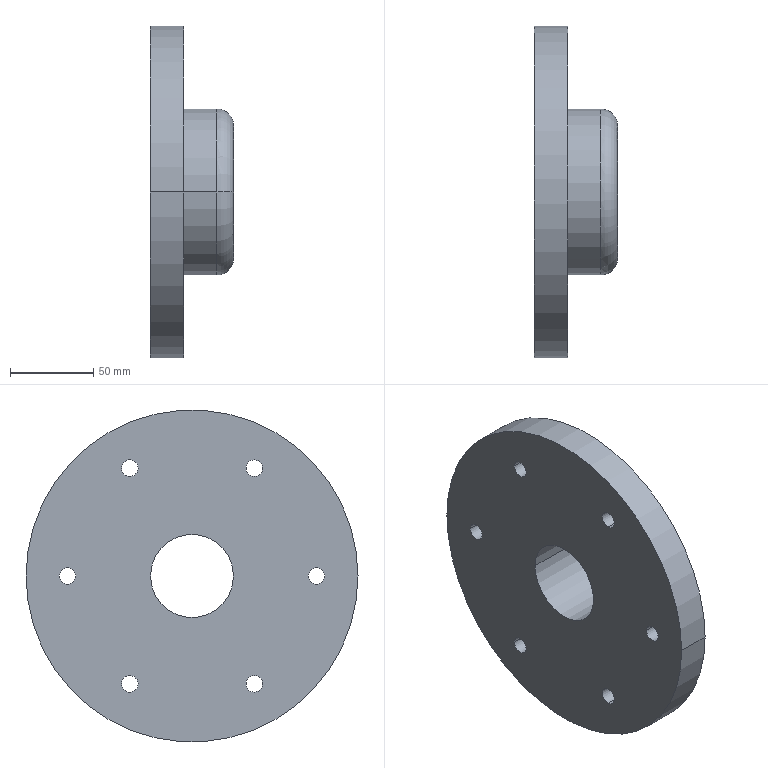Part | SolidWorks | features CirPattern 1, Fillet 1, ICE 1, Revolution 1 | 1 solid | 23 faces | box 50 x 200 x 200 mm | volume 749898 mm3 | cylinder 18 | plane 3 | torus 2 | commonest cylinder face diameters 10 x12 50 x2 100 x2 200 x2
STEP:
#1=CARTESIAN_POINT('',(40.,-50.,0.));
#2=VERTEX_POINT('',#1);
#3=CARTESIAN_POINT('',(40.,50.,0.));
#4=VERTEX_POINT('',#3);
#5=CARTESIAN_POINT('',(40.,0.,0.));
#6=DIRECTION('',(-1.,0.,0.));
#7=DIRECTION('',(0.,1.,0.));
#8=AXIS2_PLACEMENT_3D('',#5,#6,#7);
#9=CIRCLE('',#8,50.);
#10=EDGE_CURVE('',#2,#4,#9,.T.);
#11=ORIENTED_EDGE('',*,*,#10,.F.);
#12=CARTESIAN_POINT('',(50.,-40.,0.));
#13=VERTEX_POINT('',#12);
#14=CARTESIAN_POINT('',(40.,-40.,0.));
#15=DIRECTION('',(0.,0.,1.));
#16=DIRECTION('',(0.,-1.,0.));
#17=AXIS2_PLACEMENT_3D('',#14,#15,#16);
#18=CIRCLE('',#17,10.);
#19=EDGE_CURVE('',#2,#13,#18,.T.);
#20=ORIENTED_EDGE('',*,*,#19,.T.);
#21=CARTESIAN_POINT('',(50.,40.,0.));
#22=VERTEX_POINT('',#21);
#23=CARTESIAN_POINT('',(50.,0.,0.));
#24=DIRECTION('',(1.,0.,0.));
#25=DIRECTION('',(0.,1.,0.));
#26=AXIS2_PLACEMENT_3D('',#23,#24,#25);
#27=CIRCLE('',#26,40.);
#28=EDGE_CURVE('',#22,#13,#27,.T.);
#29=ORIENTED_EDGE('',*,*,#28,.F.);
#30=CARTESIAN_POINT('',(40.,40.,0.));
#31=DIRECTION('',(0.,0.,-1.));
#32=DIRECTION('',(-1.,0.,0.));
#33=AXIS2_PLACEMENT_3D('',#30,#31,#32);
#34=CIRCLE('',#33,10.);
#35=EDGE_CURVE('',#4,#22,#34,.T.);
#36=ORIENTED_EDGE('',*,*,#35,.F.);
#37=EDGE_LOOP('',(#11,#20,#29,#36));
#38=FACE_OUTER_BOUND('',#37,.T.);
#39=CARTESIAN_POINT('',(40.,0.,0.));
#40=DIRECTION('',(1.,0.,0.));
#41=DIRECTION('',(0.,1.,0.));
#42=AXIS2_PLACEMENT_3D('',#39,#40,#41);
#43=TOROIDAL_SURFACE('',#42,40.,10.);
#44=ADVANCED_FACE('',(#38),#43,.T.);
#45=CARTESIAN_POINT('',(0.,32.5,-64.952));
#46=VERTEX_POINT('',#45);
#47=CARTESIAN_POINT('',(0.,42.5,-64.952));
#48=VERTEX_POINT('',#47);
#49=CARTESIAN_POINT('',(0.,37.5,-64.952));
#50=DIRECTION('',(1.,0.,0.));
#51=DIRECTION('',(0.,-1.,0.));
#52=AXIS2_PLACEMENT_3D('',#49,#50,#51);
#53=CIRCLE('',#52,5.);
#54=EDGE_CURVE('',#46,#48,#53,.T.);
#55=ORIENTED_EDGE('',*,*,#54,.F.);
#56=CARTESIAN_POINT('',(20.,32.5,-64.952));
#57=VERTEX_POINT('',#56);
#58=CARTESIAN_POINT('',(-0.001,32.5,-64.952));
#59=DIRECTION('',(1.,0.,0.));
#60=VECTOR('',#59,1000.);
#61=LINE('',#58,#60);
#62=EDGE_CURVE('',#46,#57,#61,.T.);
#63=ORIENTED_EDGE('',*,*,#62,.T.);
#64=CARTESIAN_POINT('',(20.,42.5,-64.952));
#65=VERTEX_POINT('',#64);
#66=CARTESIAN_POINT('',(20.,37.5,-64.952));
#67=DIRECTION('',(1.,0.,0.));
#68=DIRECTION('',(0.,0.5,-0.866));
#69=AXIS2_PLACEMENT_3D('',#66,#67,#68);
#70=CIRCLE('',#69,5.);
#71=EDGE_CURVE('',#57,#65,#70,.T.);
#72=ORIENTED_EDGE('',*,*,#71,.T.);
#73=CARTESIAN_POINT('',(-0.001,42.5,-64.952));
#74=DIRECTION('',(1.,0.,0.));
#75=VECTOR('',#74,1000.);
#76=LINE('',#73,#75);
#77=EDGE_CURVE('',#48,#65,#76,.T.);
#78=ORIENTED_EDGE('',*,*,#77,.F.);
#79=EDGE_LOOP('',(#55,#63,#72,#78));
#80=FACE_OUTER_BOUND('',#79,.T.);
#81=CARTESIAN_POINT('',(-0.001,37.5,-64.952));
#82=DIRECTION('',(1.,0.,0.));
#83=DIRECTION('',(0.,1.,0.));
#84=AXIS2_PLACEMENT_3D('',#81,#82,#83);
#85=CYLINDRICAL_SURFACE('',#84,5.);
#86=ADVANCED_FACE('',(#80),#85,.F.);
#87=CARTESIAN_POINT('',(0.,-37.5,-59.952));
#88=VERTEX_POINT('',#87);
#89=CARTESIAN_POINT('',(0.,-37.5,-69.952));
#90=VERTEX_POINT('',#89);
#91=CARTESIAN_POINT('',(0.,-37.5,-64.952));
#92=DIRECTION('',(1.,0.,0.));
#93=DIRECTION('',(0.,-1.,0.));
#94=AXIS2_PLACEMENT_3D('',#91,#92,#93);
#95=CIRCLE('',#94,5.);
#96=EDGE_CURVE('',#88,#90,#95,.T.);
#97=ORIENTED_EDGE('',*,*,#96,.F.);
#98=CARTESIAN_POINT('',(20.,-37.5,-59.952));
#99=VERTEX_POINT('',#98);
#100=CARTESIAN_POINT('',(-0.001,-37.5,-59.952));
#101=DIRECTION('',(1.,0.,0.));
#102=VECTOR('',#101,1000.);
#103=LINE('',#100,#102);
#104=EDGE_CURVE('',#88,#99,#103,.T.);
#105=ORIENTED_EDGE('',*,*,#104,.T.);
#106=CARTESIAN_POINT('',(20.,-37.5,-69.952));
#107=VERTEX_POINT('',#106);
#108=CARTESIAN_POINT('',(20.,-37.5,-64.952));
#109=DIRECTION('',(1.,0.,0.));
#110=DIRECTION('',(0.,-0.5,-0.866));
#111=AXIS2_PLACEMENT_3D('',#108,#109,#110);
#112=CIRCLE('',#111,5.);
#113=EDGE_CURVE('',#99,#107,#112,.T.);
#114=ORIENTED_EDGE('',*,*,#113,.T.);
#115=CARTESIAN_POINT('',(-0.001,-37.5,-69.952));
#116=DIRECTION('',(1.,0.,0.));
#117=VECTOR('',#116,1000.);
#118=LINE('',#115,#117);
#119=EDGE_CURVE('',#90,#107,#118,.T.);
#120=ORIENTED_EDGE('',*,*,#119,.F.);
#121=EDGE_LOOP('',(#97,#105,#114,#120));
#122=FACE_OUTER_BOUND('',#121,.T.);
#123=CARTESIAN_POINT('',(-0.001,-37.5,-64.952));
#124=DIRECTION('',(1.,0.,0.));
#125=DIRECTION('',(0.,0.,-1.));
#126=AXIS2_PLACEMENT_3D('',#123,#124,#125);
#127=CYLINDRICAL_SURFACE('',#126,5.);
#128=ADVANCED_FACE('',(#122),#127,.F.);
#129=CARTESIAN_POINT('',(0.,-80.,0.));
#130=VERTEX_POINT('',#129);
#131=CARTESIAN_POINT('',(0.,-70.,0.));
#132=VERTEX_POINT('',#131);
#133=CARTESIAN_POINT('',(0.,-75.,0.));
#134=DIRECTION('',(1.,0.,0.));
#135=DIRECTION('',(0.,-1.,0.));
#136=AXIS2_PLACEMENT_3D('',#133,#134,#135);
#137=CIRCLE('',#136,5.);
#138=EDGE_CURVE('',#130,#132,#137,.T.);
#139=ORIENTED_EDGE('',*,*,#138,.F.);
#140=CARTESIAN_POINT('',(20.,-80.,0.));
#141=VERTEX_POINT('',#140);
#142=CARTESIAN_POINT('',(-0.001,-80.,0.));
#143=DIRECTION('',(1.,0.,0.));
#144=VECTOR('',#143,1000.);
#145=LINE('',#142,#144);
#146=EDGE_CURVE('',#130,#141,#145,.T.);
#147=ORIENTED_EDGE('',*,*,#146,.T.);
#148=CARTESIAN_POINT('',(20.,-70.,0.));
#149=VERTEX_POINT('',#148);
#150=CARTESIAN_POINT('',(20.,-75.,0.));
#151=DIRECTION('',(1.,0.,0.));
#152=DIRECTION('',(0.,-1.,0.));
#153=AXIS2_PLACEMENT_3D('',#150,#151,#152);
#154=CIRCLE('',#153,5.);
#155=EDGE_CURVE('',#141,#149,#154,.T.);
#156=ORIENTED_EDGE('',*,*,#155,.T.);
#157=CARTESIAN_POINT('',(-0.001,-70.,0.));
#158=DIRECTION('',(1.,0.,0.));
#159=VECTOR('',#158,1000.);
#160=LINE('',#157,#159);
#161=EDGE_CURVE('',#132,#149,#160,.T.);
#162=ORIENTED_EDGE('',*,*,#161,.F.);
#163=EDGE_LOOP('',(#139,#147,#156,#162));
#164=FACE_OUTER_BOUND('',#163,.T.);
#165=CARTESIAN_POINT('',(-0.001,-75.,0.));
#166=DIRECTION('',(1.,0.,0.));
#167=DIRECTION('',(0.,1.,0.));
#168=AXIS2_PLACEMENT_3D('',#165,#166,#167);
#169=CYLINDRICAL_SURFACE('',#168,5.);
#170=ADVANCED_FACE('',(#164),#169,.F.);
#171=CARTESIAN_POINT('',(0.,-37.5,69.952));
#172=VERTEX_POINT('',#171);
#173=CARTESIAN_POINT('',(0.,-37.5,59.952));
#174=VERTEX_POINT('',#173);
#175=CARTESIAN_POINT('',(0.,-37.5,64.952));
#176=DIRECTION('',(1.,0.,0.));
#177=DIRECTION('',(0.,-1.,0.));
#178=AXIS2_PLACEMENT_3D('',#175,#176,#177);
#179=CIRCLE('',#178,5.);
#180=EDGE_CURVE('',#172,#174,#179,.T.);
#181=ORIENTED_EDGE('',*,*,#180,.F.);
#182=CARTESIAN_POINT('',(20.,-37.5,69.952));
#183=VERTEX_POINT('',#182);
#184=CARTESIAN_POINT('',(-0.001,-37.5,69.952));
#185=DIRECTION('',(1.,0.,0.));
#186=VECTOR('',#185,1000.);
#187=LINE('',#184,#186);
#188=EDGE_CURVE('',#172,#183,#187,.T.);
#189=ORIENTED_EDGE('',*,*,#188,.T.);
#190=CARTESIAN_POINT('',(20.,-37.5,59.952));
#191=VERTEX_POINT('',#190);
#192=CARTESIAN_POINT('',(20.,-37.5,64.952));
#193=DIRECTION('',(1.,0.,0.));
#194=DIRECTION('',(0.,-0.5,0.866));
#195=AXIS2_PLACEMENT_3D('',#192,#193,#194);
#196=CIRCLE('',#195,5.);
#197=EDGE_CURVE('',#183,#191,#196,.T.);
#198=ORIENTED_EDGE('',*,*,#197,.T.);
#199=CARTESIAN_POINT('',(-0.001,-37.5,59.952));
#200=DIRECTION('',(1.,0.,0.));
#201=VECTOR('',#200,1000.);
#202=LINE('',#199,#201);
#203=EDGE_CURVE('',#174,#191,#202,.T.);
#204=ORIENTED_EDGE('',*,*,#203,.F.);
#205=EDGE_LOOP('',(#181,#189,#198,#204));
#206=FACE_OUTER_BOUND('',#205,.T.);
#207=CARTESIAN_POINT('',(-0.001,-37.5,64.952));
#208=DIRECTION('',(1.,0.,0.));
#209=DIRECTION('',(0.,0.,-1.));
#210=AXIS2_PLACEMENT_3D('',#207,#208,#209);
#211=CYLINDRICAL_SURFACE('',#210,5.);
#212=ADVANCED_FACE('',(#206),#211,.F.);
#213=CARTESIAN_POINT('',(0.,32.5,64.952));
#214=VERTEX_POINT('',#213);
#215=CARTESIAN_POINT('',(0.,42.5,64.952));
#216=VERTEX_POINT('',#215);
#217=CARTESIAN_POINT('',(0.,37.5,64.952));
#218=DIRECTION('',(1.,0.,0.));
#219=DIRECTION('',(0.,-1.,0.));
#220=AXIS2_PLACEMENT_3D('',#217,#218,#219);
#221=CIRCLE('',#220,5.);
#222=EDGE_CURVE('',#214,#216,#221,.T.);
#223=ORIENTED_EDGE('',*,*,#222,.F.);
#224=CARTESIAN_POINT('',(20.,32.5,64.952));
#225=VERTEX_POINT('',#224);
#226=CARTESIAN_POINT('',(-0.001,32.5,64.952));
#227=DIRECTION('',(1.,0.,0.));
#228=VECTOR('',#227,1000.);
#229=LINE('',#226,#228);
#230=EDGE_CURVE('',#214,#225,#229,.T.);
#231=ORIENTED_EDGE('',*,*,#230,.T.);
#232=CARTESIAN_POINT('',(20.,42.5,64.952));
#233=VERTEX_POINT('',#232);
#234=CARTESIAN_POINT('',(20.,37.5,64.952));
#235=DIRECTION('',(1.,0.,0.));
#236=DIRECTION('',(0.,0.5,0.866));
#237=AXIS2_PLACEMENT_3D('',#234,#235,#236);
#238=CIRCLE('',#237,5.);
#239=EDGE_CURVE('',#225,#233,#238,.T.);
#240=ORIENTED_EDGE('',*,*,#239,.T.);
#241=CARTESIAN_POINT('',(-0.001,42.5,64.952));
#242=DIRECTION('',(1.,0.,0.));
#243=VECTOR('',#242,1000.);
#244=LINE('',#241,#243);
#245=EDGE_CURVE('',#216,#233,#244,.T.);
#246=ORIENTED_EDGE('',*,*,#245,.F.);
#247=EDGE_LOOP('',(#223,#231,#240,#246));
#248=FACE_OUTER_BOUND('',#247,.T.);
#249=CARTESIAN_POINT('',(-0.001,37.5,64.952));
#250=DIRECTION('',(1.,0.,0.));
#251=DIRECTION('',(0.,1.,0.));
#252=AXIS2_PLACEMENT_3D('',#249,#250,#251);
#253=CYLINDRICAL_SURFACE('',#252,5.);
#254=ADVANCED_FACE('',(#248),#253,.F.);
#255=CARTESIAN_POINT('',(0.,70.,0.));
#256=VERTEX_POINT('',#255);
#257=CARTESIAN_POINT('',(0.,80.,0.));
#258=VERTEX_POINT('',#257);
#259=CARTESIAN_POINT('',(0.,75.,0.));
#260=DIRECTION('',(1.,0.,0.));
#261=DIRECTION('',(0.,-1.,0.));
#262=AXIS2_PLACEMENT_3D('',#259,#260,#261);
#263=CIRCLE('',#262,5.);
#264=EDGE_CURVE('',#256,#258,#263,.T.);
#265=ORIENTED_EDGE('',*,*,#264,.F.);
#266=CARTESIAN_POINT('',(20.,70.,0.));
#267=VERTEX_POINT('',#266);
#268=CARTESIAN_POINT('',(-0.001,70.,0.));
#269=DIRECTION('',(1.,0.,0.));
#270=VECTOR('',#269,1000.);
#271=LINE('',#268,#270);
#272=EDGE_CURVE('',#256,#267,#271,.T.);
#273=ORIENTED_EDGE('',*,*,#272,.T.);
#274=CARTESIAN_POINT('',(20.,80.,0.));
#275=VERTEX_POINT('',#274);
#276=CARTESIAN_POINT('',(20.,75.,0.));
#277=DIRECTION('',(1.,0.,0.));
#278=DIRECTION('',(0.,1.,0.));
#279=AXIS2_PLACEMENT_3D('',#276,#277,#278);
#280=CIRCLE('',#279,5.);
#281=EDGE_CURVE('',#267,#275,#280,.T.);
#282=ORIENTED_EDGE('',*,*,#281,.T.);
#283=CARTESIAN_POINT('',(-0.001,80.,0.));
#284=DIRECTION('',(1.,0.,0.));
#285=VECTOR('',#284,1000.);
#286=LINE('',#283,#285);
#287=EDGE_CURVE('',#258,#275,#286,.T.);
#288=ORIENTED_EDGE('',*,*,#287,.F.);
#289=EDGE_LOOP('',(#265,#273,#282,#288));
#290=FACE_OUTER_BOUND('',#289,.T.);
#291=CARTESIAN_POINT('',(-0.001,75.,0.));
#292=DIRECTION('',(1.,0.,0.));
#293=DIRECTION('',(0.,1.,0.));
#294=AXIS2_PLACEMENT_3D('',#291,#292,#293);
#295=CYLINDRICAL_SURFACE('',#294,5.);
#296=ADVANCED_FACE('',(#290),#295,.F.);
#297=CARTESIAN_POINT('',(0.,-25.,0.));
#298=VERTEX_POINT('',#297);
#299=CARTESIAN_POINT('',(0.,25.,0.));
#300=VERTEX_POINT('',#299);
#301=CARTESIAN_POINT('',(0.,0.,0.));
#302=DIRECTION('',(1.,0.,0.));
#303=DIRECTION('',(0.,1.,0.));
#304=AXIS2_PLACEMENT_3D('',#301,#302,#303);
#305=CIRCLE('',#304,25.);
#306=EDGE_CURVE('',#298,#300,#305,.T.);
#307=ORIENTED_EDGE('',*,*,#306,.F.);
#308=CARTESIAN_POINT('',(50.,-25.,0.));
#309=VERTEX_POINT('',#308);
#310=CARTESIAN_POINT('',(113.214,-25.,0.));
#311=DIRECTION('',(1.,0.,0.));
#312=VECTOR('',#311,1000.);
#313=LINE('',#310,#312);
#314=EDGE_CURVE('',#298,#309,#313,.T.);
#315=ORIENTED_EDGE('',*,*,#314,.T.);
#316=CARTESIAN_POINT('',(50.,25.,0.));
#317=VERTEX_POINT('',#316);
#318=CARTESIAN_POINT('',(50.,0.,0.));
#319=DIRECTION('',(1.,0.,0.));
#320=DIRECTION('',(0.,1.,0.));
#321=AXIS2_PLACEMENT_3D('',#318,#319,#320);
#322=CIRCLE('',#321,25.);
#323=EDGE_CURVE('',#309,#317,#322,.T.);
#324=ORIENTED_EDGE('',*,*,#323,.T.);
#325=CARTESIAN_POINT('',(113.214,25.,0.));
#326=DIRECTION('',(1.,0.,0.));
#327=VECTOR('',#326,1000.);
#328=LINE('',#325,#327);
#329=EDGE_CURVE('',#300,#317,#328,.T.);
#330=ORIENTED_EDGE('',*,*,#329,.F.);
#331=EDGE_LOOP('',(#307,#315,#324,#330));
#332=FACE_OUTER_BOUND('',#331,.T.);
#333=CARTESIAN_POINT('',(113.214,0.,0.));
#334=DIRECTION('',(1.,0.,0.));
#335=DIRECTION('',(0.,1.,0.));
#336=AXIS2_PLACEMENT_3D('',#333,#334,#335);
#337=CYLINDRICAL_SURFACE('',#336,25.);
#338=ADVANCED_FACE('',(#332),#337,.F.);
#339=CARTESIAN_POINT('',(20.,50.,0.));
#340=VERTEX_POINT('',#339);
#341=CARTESIAN_POINT('',(20.,-50.,0.));
#342=VERTEX_POINT('',#341);
#343=CARTESIAN_POINT('',(20.,0.,0.));
#344=DIRECTION('',(1.,0.,0.));
#345=DIRECTION('',(0.,1.,0.));
#346=AXIS2_PLACEMENT_3D('',#343,#344,#345);
#347=CIRCLE('',#346,50.);
#348=EDGE_CURVE('',#340,#342,#347,.T.);
#349=ORIENTED_EDGE('',*,*,#348,.T.);
#350=CARTESIAN_POINT('',(113.214,-50.,0.));
#351=DIRECTION('',(1.,0.,0.));
#352=VECTOR('',#351,1000.);
#353=LINE('',#350,#352);
#354=EDGE_CURVE('',#342,#2,#353,.T.);
#355=ORIENTED_EDGE('',*,*,#354,.T.);
#356=ORIENTED_EDGE('',*,*,#10,.T.);
#357=CARTESIAN_POINT('',(113.214,50.,0.));
#358=DIRECTION('',(1.,0.,0.));
#359=VECTOR('',#358,1000.);
#360=LINE('',#357,#359);
#361=EDGE_CURVE('',#340,#4,#360,.T.);
#362=ORIENTED_EDGE('',*,*,#361,.F.);
#363=EDGE_LOOP('',(#349,#355,#356,#362));
#364=FACE_OUTER_BOUND('',#363,.T.);
#365=CARTESIAN_POINT('',(113.214,0.,0.));
#366=DIRECTION('',(1.,0.,0.));
#367=DIRECTION('',(0.,1.,0.));
#368=AXIS2_PLACEMENT_3D('',#365,#366,#367);
#369=CYLINDRICAL_SURFACE('',#368,50.);
#370=ADVANCED_FACE('',(#364),#369,.T.);
#371=CARTESIAN_POINT('',(0.,100.,0.));
#372=VERTEX_POINT('',#371);
#373=CARTESIAN_POINT('',(0.,-100.,0.));
#374=VERTEX_POINT('',#373);
#375=CARTESIAN_POINT('',(0.,0.,0.));
#376=DIRECTION('',(1.,0.,0.));
#377=DIRECTION('',(0.,1.,0.));
#378=AXIS2_PLACEMENT_3D('',#375,#376,#377);
#379=CIRCLE('',#378,100.);
#380=EDGE_CURVE('',#372,#374,#379,.T.);
#381=ORIENTED_EDGE('',*,*,#380,.T.);
#382=CARTESIAN_POINT('',(20.,-100.,0.));
#383=VERTEX_POINT('',#382);
#384=CARTESIAN_POINT('',(113.214,-100.,0.));
#385=DIRECTION('',(1.,0.,0.));
#386=VECTOR('',#385,1000.);
#387=LINE('',#384,#386);
#388=EDGE_CURVE('',#374,#383,#387,.T.);
#389=ORIENTED_EDGE('',*,*,#388,.T.);
#390=CARTESIAN_POINT('',(20.,100.,0.));
#391=VERTEX_POINT('',#390);
#392=CARTESIAN_POINT('',(20.,0.,0.));
#393=DIRECTION('',(1.,0.,0.));
#394=DIRECTION('',(0.,1.,0.));
#395=AXIS2_PLACEMENT_3D('',#392,#393,#394);
#396=CIRCLE('',#395,100.);
#397=EDGE_CURVE('',#391,#383,#396,.T.);
#398=ORIENTED_EDGE('',*,*,#397,.F.);
#399=CARTESIAN_POINT('',(113.214,100.,0.));
#400=DIRECTION('',(1.,0.,0.));
#401=VECTOR('',#400,1000.);
#402=LINE('',#399,#401);
#403=EDGE_CURVE('',#372,#391,#402,.T.);
#404=ORIENTED_EDGE('',*,*,#403,.F.);
#405=EDGE_LOOP('',(#381,#389,#398,#404));
#406=FACE_OUTER_BOUND('',#405,.T.);
#407=CARTESIAN_POINT('',(113.214,0.,0.));
#408=DIRECTION('',(1.,0.,0.));
#409=DIRECTION('',(0.,1.,0.));
#410=AXIS2_PLACEMENT_3D('',#407,#408,#409);
#411=CYLINDRICAL_SURFACE('',#410,100.);
#412=ADVANCED_FACE('',(#406),#411,.T.);
#413=ORIENTED_EDGE('',*,*,#388,.F.);
#414=CARTESIAN_POINT('',(0.,0.,0.));
#415=DIRECTION('',(1.,0.,0.));
#416=DIRECTION('',(0.,1.,0.));
#417=AXIS2_PLACEMENT_3D('',#414,#415,#416);
#418=CIRCLE('',#417,100.);
#419=EDGE_CURVE('',#374,#372,#418,.T.);
#420=ORIENTED_EDGE('',*,*,#419,.T.);
#421=ORIENTED_EDGE('',*,*,#403,.T.);
#422=CARTESIAN_POINT('',(20.,0.,0.));
#423=DIRECTION('',(1.,0.,0.));
#424=DIRECTION('',(0.,1.,0.));
#425=AXIS2_PLACEMENT_3D('',#422,#423,#424);
#426=CIRCLE('',#425,100.);
#427=EDGE_CURVE('',#383,#391,#426,.T.);
#428=ORIENTED_EDGE('',*,*,#427,.F.);
#429=EDGE_LOOP('',(#413,#420,#421,#428));
#430=FACE_OUTER_BOUND('',#429,.T.);
#431=CARTESIAN_POINT('',(113.214,0.,0.));
#432=DIRECTION('',(1.,0.,0.));
#433=DIRECTION('',(0.,1.,0.));
#434=AXIS2_PLACEMENT_3D('',#431,#432,#433);
#435=CYLINDRICAL_SURFACE('',#434,100.);
#436=ADVANCED_FACE('',(#430),#435,.T.);
#437=CARTESIAN_POINT('',(20.,37.5,-64.952));
#438=DIRECTION('',(1.,0.,0.));
#439=DIRECTION('',(0.,0.5,-0.866));
#440=AXIS2_PLACEMENT_3D('',#437,#438,#439);
#441=CIRCLE('',#440,5.);
#442=EDGE_CURVE('',#65,#57,#441,.T.);
#443=ORIENTED_EDGE('',*,*,#442,.F.);
#444=ORIENTED_EDGE('',*,*,#71,.F.);
#445=EDGE_LOOP('',(#443,#444));
#446=FACE_BOUND('',#445,.T.);
#447=CARTESIAN_POINT('',(20.,-37.5,-64.952));
#448=DIRECTION('',(1.,0.,0.));
#449=DIRECTION('',(0.,-0.5,-0.866));
#450=AXIS2_PLACEMENT_3D('',#447,#448,#449);
#451=CIRCLE('',#450,5.);
#452=EDGE_CURVE('',#107,#99,#451,.T.);
#453=ORIENTED_EDGE('',*,*,#452,.F.);
#454=ORIENTED_EDGE('',*,*,#113,.F.);
#455=EDGE_LOOP('',(#453,#454));
#456=FACE_BOUND('',#455,.T.);
#457=CARTESIAN_POINT('',(20.,-75.,0.));
#458=DIRECTION('',(1.,0.,0.));
#459=DIRECTION('',(0.,-1.,0.));
#460=AXIS2_PLACEMENT_3D('',#457,#458,#459);
#461=CIRCLE('',#460,5.);
#462=EDGE_CURVE('',#149,#141,#461,.T.);
#463=ORIENTED_EDGE('',*,*,#462,.F.);
#464=ORIENTED_EDGE('',*,*,#155,.F.);
#465=EDGE_LOOP('',(#463,#464));
#466=FACE_BOUND('',#465,.T.);
#467=CARTESIAN_POINT('',(20.,-37.5,64.952));
#468=DIRECTION('',(1.,0.,0.));
#469=DIRECTION('',(0.,-0.5,0.866));
#470=AXIS2_PLACEMENT_3D('',#467,#468,#469);
#471=CIRCLE('',#470,5.);
#472=EDGE_CURVE('',#191,#183,#471,.T.);
#473=ORIENTED_EDGE('',*,*,#472,.F.);
#474=ORIENTED_EDGE('',*,*,#197,.F.);
#475=EDGE_LOOP('',(#473,#474));
#476=FACE_BOUND('',#475,.T.);
#477=CARTESIAN_POINT('',(20.,37.5,64.952));
#478=DIRECTION('',(1.,0.,0.));
#479=DIRECTION('',(0.,0.5,0.866));
#480=AXIS2_PLACEMENT_3D('',#477,#478,#479);
#481=CIRCLE('',#480,5.);
#482=EDGE_CURVE('',#233,#225,#481,.T.);
#483=ORIENTED_EDGE('',*,*,#482,.F.);
#484=ORIENTED_EDGE('',*,*,#239,.F.);
#485=EDGE_LOOP('',(#483,#484));
#486=FACE_BOUND('',#485,.T.);
#487=CARTESIAN_POINT('',(20.,75.,0.));
#488=DIRECTION('',(1.,0.,0.));
#489=DIRECTION('',(0.,1.,0.));
#490=AXIS2_PLACEMENT_3D('',#487,#488,#489);
#491=CIRCLE('',#490,5.);
#492=EDGE_CURVE('',#275,#267,#491,.T.);
#493=ORIENTED_EDGE('',*,*,#492,.F.);
#494=ORIENTED_EDGE('',*,*,#281,.F.);
#495=EDGE_LOOP('',(#493,#494));
#496=FACE_BOUND('',#495,.T.);
#497=ORIENTED_EDGE('',*,*,#397,.T.);
#498=ORIENTED_EDGE('',*,*,#427,.T.);
#499=EDGE_LOOP('',(#497,#498));
#500=FACE_OUTER_BOUND('',#499,.T.);
#501=ORIENTED_EDGE('',*,*,#348,.F.);
#502=CARTESIAN_POINT('',(20.,0.,0.));
#503=DIRECTION('',(1.,0.,0.));
#504=DIRECTION('',(0.,1.,0.));
#505=AXIS2_PLACEMENT_3D('',#502,#503,#504);
#506=CIRCLE('',#505,50.);
#507=EDGE_CURVE('',#342,#340,#506,.T.);
#508=ORIENTED_EDGE('',*,*,#507,.F.);
#509=EDGE_LOOP('',(#501,#508));
#510=FACE_BOUND('',#509,.T.);
#511=CARTESIAN_POINT('',(20.,100.,0.));
#512=DIRECTION('',(1.,0.,0.));
#513=DIRECTION('',(0.,1.,0.));
#514=AXIS2_PLACEMENT_3D('',#511,#512,#513);
#515=PLANE('',#514);
#516=ADVANCED_FACE('',(#446,#456,#466,#476,#486,#496,#500,#510),#515,.T.);
#517=ORIENTED_EDGE('',*,*,#354,.F.);
#518=ORIENTED_EDGE('',*,*,#507,.T.);
#519=ORIENTED_EDGE('',*,*,#361,.T.);
#520=CARTESIAN_POINT('',(40.,0.,0.));
#521=DIRECTION('',(-1.,0.,0.));
#522=DIRECTION('',(0.,1.,0.));
#523=AXIS2_PLACEMENT_3D('',#520,#521,#522);
#524=CIRCLE('',#523,50.);
#525=EDGE_CURVE('',#4,#2,#524,.T.);
#526=ORIENTED_EDGE('',*,*,#525,.T.);
#527=EDGE_LOOP('',(#517,#518,#519,#526));
#528=FACE_OUTER_BOUND('',#527,.T.);
#529=CARTESIAN_POINT('',(113.214,0.,0.));
#530=DIRECTION('',(1.,0.,0.));
#531=DIRECTION('',(0.,1.,0.));
#532=AXIS2_PLACEMENT_3D('',#529,#530,#531);
#533=CYLINDRICAL_SURFACE('',#532,50.);
#534=ADVANCED_FACE('',(#528),#533,.T.);
#535=ORIENTED_EDGE('',*,*,#28,.T.);
#536=CARTESIAN_POINT('',(50.,0.,0.));
#537=DIRECTION('',(1.,0.,0.));
#538=DIRECTION('',(0.,1.,0.));
#539=AXIS2_PLACEMENT_3D('',#536,#537,#538);
#540=CIRCLE('',#539,40.);
#541=EDGE_CURVE('',#13,#22,#540,.T.);
#542=ORIENTED_EDGE('',*,*,#541,.T.);
#543=EDGE_LOOP('',(#535,#542));
#544=FACE_OUTER_BOUND('',#543,.T.);
#545=CARTESIAN_POINT('',(50.,0.,0.));
#546=DIRECTION('',(1.,0.,0.));
#547=DIRECTION('',(0.,1.,0.));
#548=AXIS2_PLACEMENT_3D('',#545,#546,#547);
#549=CIRCLE('',#548,25.);
#550=EDGE_CURVE('',#317,#309,#549,.T.);
#551=ORIENTED_EDGE('',*,*,#550,.F.);
#552=ORIENTED_EDGE('',*,*,#323,.F.);
#553=EDGE_LOOP('',(#551,#552));
#554=FACE_BOUND('',#553,.T.);
#555=CARTESIAN_POINT('',(50.,50.,0.));
#556=DIRECTION('',(1.,0.,0.));
#557=DIRECTION('',(0.,1.,0.));
#558=AXIS2_PLACEMENT_3D('',#555,#556,#557);
#559=PLANE('',#558);
#560=ADVANCED_FACE('',(#544,#554),#559,.T.);
#561=ORIENTED_EDGE('',*,*,#314,.F.);
#562=CARTESIAN_POINT('',(0.,0.,0.));
#563=DIRECTION('',(1.,0.,0.));
#564=DIRECTION('',(0.,1.,0.));
#565=AXIS2_PLACEMENT_3D('',#562,#563,#564);
#566=CIRCLE('',#565,25.);
#567=EDGE_CURVE('',#300,#298,#566,.T.);
#568=ORIENTED_EDGE('',*,*,#567,.F.);
#569=ORIENTED_EDGE('',*,*,#329,.T.);
#570=ORIENTED_EDGE('',*,*,#550,.T.);
#571=EDGE_LOOP('',(#561,#568,#569,#570));
#572=FACE_OUTER_BOUND('',#571,.T.);
#573=CARTESIAN_POINT('',(113.214,0.,0.));
#574=DIRECTION('',(1.,0.,0.));
#575=DIRECTION('',(0.,1.,0.));
#576=AXIS2_PLACEMENT_3D('',#573,#574,#575);
#577=CYLINDRICAL_SURFACE('',#576,25.);
#578=ADVANCED_FACE('',(#572),#577,.F.);
#579=CARTESIAN_POINT('',(0.,37.5,-64.952));
#580=DIRECTION('',(1.,0.,0.));
#581=DIRECTION('',(0.,-1.,0.));
#582=AXIS2_PLACEMENT_3D('',#579,#580,#581);
#583=CIRCLE('',#582,5.);
#584=EDGE_CURVE('',#48,#46,#583,.T.);
#585=ORIENTED_EDGE('',*,*,#584,.T.);
#586=ORIENTED_EDGE('',*,*,#54,.T.);
#587=EDGE_LOOP('',(#585,#586));
#588=FACE_BOUND('',#587,.T.);
#589=CARTESIAN_POINT('',(0.,-37.5,-64.952));
#590=DIRECTION('',(1.,0.,0.));
#591=DIRECTION('',(0.,-1.,0.));
#592=AXIS2_PLACEMENT_3D('',#589,#590,#591);
#593=CIRCLE('',#592,5.);
#594=EDGE_CURVE('',#90,#88,#593,.T.);
#595=ORIENTED_EDGE('',*,*,#594,.T.);
#596=ORIENTED_EDGE('',*,*,#96,.T.);
#597=EDGE_LOOP('',(#595,#596));
#598=FACE_BOUND('',#597,.T.);
#599=CARTESIAN_POINT('',(0.,-75.,0.));
#600=DIRECTION('',(1.,0.,0.));
#601=DIRECTION('',(0.,-1.,0.));
#602=AXIS2_PLACEMENT_3D('',#599,#600,#601);
#603=CIRCLE('',#602,5.);
#604=EDGE_CURVE('',#132,#130,#603,.T.);
#605=ORIENTED_EDGE('',*,*,#604,.T.);
#606=ORIENTED_EDGE('',*,*,#138,.T.);
#607=EDGE_LOOP('',(#605,#606));
#608=FACE_BOUND('',#607,.T.);
#609=CARTESIAN_POINT('',(0.,-37.5,64.952));
#610=DIRECTION('',(1.,0.,0.));
#611=DIRECTION('',(0.,-1.,0.));
#612=AXIS2_PLACEMENT_3D('',#609,#610,#611);
#613=CIRCLE('',#612,5.);
#614=EDGE_CURVE('',#174,#172,#613,.T.);
#615=ORIENTED_EDGE('',*,*,#614,.T.);
#616=ORIENTED_EDGE('',*,*,#180,.T.);
#617=EDGE_LOOP('',(#615,#616));
#618=FACE_BOUND('',#617,.T.);
#619=CARTESIAN_POINT('',(0.,37.5,64.952));
#620=DIRECTION('',(1.,0.,0.));
#621=DIRECTION('',(0.,-1.,0.));
#622=AXIS2_PLACEMENT_3D('',#619,#620,#621);
#623=CIRCLE('',#622,5.);
#624=EDGE_CURVE('',#216,#214,#623,.T.);
#625=ORIENTED_EDGE('',*,*,#624,.T.);
#626=ORIENTED_EDGE('',*,*,#222,.T.);
#627=EDGE_LOOP('',(#625,#626));
#628=FACE_BOUND('',#627,.T.);
#629=CARTESIAN_POINT('',(0.,75.,0.));
#630=DIRECTION('',(1.,0.,0.));
#631=DIRECTION('',(0.,-1.,0.));
#632=AXIS2_PLACEMENT_3D('',#629,#630,#631);
#633=CIRCLE('',#632,5.);
#634=EDGE_CURVE('',#258,#256,#633,.T.);
#635=ORIENTED_EDGE('',*,*,#634,.T.);
#636=ORIENTED_EDGE('',*,*,#264,.T.);
#637=EDGE_LOOP('',(#635,#636));
#638=FACE_BOUND('',#637,.T.);
#639=ORIENTED_EDGE('',*,*,#567,.T.);
#640=ORIENTED_EDGE('',*,*,#306,.T.);
#641=EDGE_LOOP('',(#639,#640));
#642=FACE_BOUND('',#641,.T.);
#643=ORIENTED_EDGE('',*,*,#380,.F.);
#644=ORIENTED_EDGE('',*,*,#419,.F.);
#645=EDGE_LOOP('',(#643,#644));
#646=FACE_OUTER_BOUND('',#645,.T.);
#647=CARTESIAN_POINT('',(0.,25.,0.));
#648=DIRECTION('',(-1.,0.,0.));
#649=DIRECTION('',(0.,-1.,0.));
#650=AXIS2_PLACEMENT_3D('',#647,#648,#649);
#651=PLANE('',#650);
#652=ADVANCED_FACE('',(#588,#598,#608,#618,#628,#638,#642,#646),#651,.T.);
#653=ORIENTED_EDGE('',*,*,#272,.F.);
#654=ORIENTED_EDGE('',*,*,#634,.F.);
#655=ORIENTED_EDGE('',*,*,#287,.T.);
#656=ORIENTED_EDGE('',*,*,#492,.T.);
#657=EDGE_LOOP('',(#653,#654,#655,#656));
#658=FACE_OUTER_BOUND('',#657,.T.);
#659=CARTESIAN_POINT('',(-0.001,75.,0.));
#660=DIRECTION('',(1.,0.,0.));
#661=DIRECTION('',(0.,1.,0.));
#662=AXIS2_PLACEMENT_3D('',#659,#660,#661);
#663=CYLINDRICAL_SURFACE('',#662,5.);
#664=ADVANCED_FACE('',(#658),#663,.F.);
#665=ORIENTED_EDGE('',*,*,#230,.F.);
#666=ORIENTED_EDGE('',*,*,#624,.F.);
#667=ORIENTED_EDGE('',*,*,#245,.T.);
#668=ORIENTED_EDGE('',*,*,#482,.T.);
#669=EDGE_LOOP('',(#665,#666,#667,#668));
#670=FACE_OUTER_BOUND('',#669,.T.);
#671=CARTESIAN_POINT('',(-0.001,37.5,64.952));
#672=DIRECTION('',(1.,0.,0.));
#673=DIRECTION('',(0.,1.,0.));
#674=AXIS2_PLACEMENT_3D('',#671,#672,#673);
#675=CYLINDRICAL_SURFACE('',#674,5.);
#676=ADVANCED_FACE('',(#670),#675,.F.);
#677=ORIENTED_EDGE('',*,*,#188,.F.);
#678=ORIENTED_EDGE('',*,*,#614,.F.);
#679=ORIENTED_EDGE('',*,*,#203,.T.);
#680=ORIENTED_EDGE('',*,*,#472,.T.);
#681=EDGE_LOOP('',(#677,#678,#679,#680));
#682=FACE_OUTER_BOUND('',#681,.T.);
#683=CARTESIAN_POINT('',(-0.001,-37.5,64.952));
#684=DIRECTION('',(1.,0.,0.));
#685=DIRECTION('',(0.,0.,-1.));
#686=AXIS2_PLACEMENT_3D('',#683,#684,#685);
#687=CYLINDRICAL_SURFACE('',#686,5.);
#688=ADVANCED_FACE('',(#682),#687,.F.);
#689=ORIENTED_EDGE('',*,*,#146,.F.);
#690=ORIENTED_EDGE('',*,*,#604,.F.);
#691=ORIENTED_EDGE('',*,*,#161,.T.);
#692=ORIENTED_EDGE('',*,*,#462,.T.);
#693=EDGE_LOOP('',(#689,#690,#691,#692));
#694=FACE_OUTER_BOUND('',#693,.T.);
#695=CARTESIAN_POINT('',(-0.001,-75.,0.));
#696=DIRECTION('',(1.,0.,0.));
#697=DIRECTION('',(0.,1.,0.));
#698=AXIS2_PLACEMENT_3D('',#695,#696,#697);
#699=CYLINDRICAL_SURFACE('',#698,5.);
#700=ADVANCED_FACE('',(#694),#699,.F.);
#701=ORIENTED_EDGE('',*,*,#104,.F.);
#702=ORIENTED_EDGE('',*,*,#594,.F.);
#703=ORIENTED_EDGE('',*,*,#119,.T.);
#704=ORIENTED_EDGE('',*,*,#452,.T.);
#705=EDGE_LOOP('',(#701,#702,#703,#704));
#706=FACE_OUTER_BOUND('',#705,.T.);
#707=CARTESIAN_POINT('',(-0.001,-37.5,-64.952));
#708=DIRECTION('',(1.,0.,0.));
#709=DIRECTION('',(0.,0.,-1.));
#710=AXIS2_PLACEMENT_3D('',#707,#708,#709);
#711=CYLINDRICAL_SURFACE('',#710,5.);
#712=ADVANCED_FACE('',(#706),#711,.F.);
#713=ORIENTED_EDGE('',*,*,#62,.F.);
#714=ORIENTED_EDGE('',*,*,#584,.F.);
#715=ORIENTED_EDGE('',*,*,#77,.T.);
#716=ORIENTED_EDGE('',*,*,#442,.T.);
#717=EDGE_LOOP('',(#713,#714,#715,#716));
#718=FACE_OUTER_BOUND('',#717,.T.);
#719=CARTESIAN_POINT('',(-0.001,37.5,-64.952));
#720=DIRECTION('',(1.,0.,0.));
#721=DIRECTION('',(0.,1.,0.));
#722=AXIS2_PLACEMENT_3D('',#719,#720,#721);
#723=CYLINDRICAL_SURFACE('',#722,5.);
#724=ADVANCED_FACE('',(#718),#723,.F.);
#725=ORIENTED_EDGE('',*,*,#19,.F.);
#726=ORIENTED_EDGE('',*,*,#525,.F.);
#727=ORIENTED_EDGE('',*,*,#35,.T.);
#728=ORIENTED_EDGE('',*,*,#541,.F.);
#729=EDGE_LOOP('',(#725,#726,#727,#728));
#730=FACE_OUTER_BOUND('',#729,.T.);
#731=CARTESIAN_POINT('',(40.,0.,0.));
#732=DIRECTION('',(1.,0.,0.));
#733=DIRECTION('',(0.,1.,0.));
#734=AXIS2_PLACEMENT_3D('',#731,#732,#733);
#735=TOROIDAL_SURFACE('',#734,40.,10.);
#736=ADVANCED_FACE('',(#730),#735,.T.);
#737=CLOSED_SHELL('',(#44,#86,#128,#170,#212,#254,#296,#338,#370,#412,#436,#516,#534,#560,#578,#652,#664,#676,#688,#700,#712,#724,#736));
#738=MANIFOLD_SOLID_BREP('',#737);
#739=CARTESIAN_POINT('',(0.,0.,0.));
#740=DIRECTION('',(0.,0.,1.));
#741=DIRECTION('',(1.,0.,0.));
#742=AXIS2_PLACEMENT_3D('',#739,#740,#741);
#743=(LENGTH_UNIT()NAMED_UNIT(*)SI_UNIT(.MILLI.,.METRE.));
#744=UNCERTAINTY_MEASURE_WITH_UNIT(LENGTH_MEASURE(0.00001),#743,'','');
#745=(NAMED_UNIT(*)PLANE_ANGLE_UNIT()SI_UNIT($,.RADIAN.));
#746=(NAMED_UNIT(*)SI_UNIT($,.STERADIAN.)SOLID_ANGLE_UNIT());
#747=(GEOMETRIC_REPRESENTATION_CONTEXT(3)GLOBAL_UNCERTAINTY_ASSIGNED_CONTEXT((#744))GLOBAL_UNIT_ASSIGNED_CONTEXT((#743,#745,#746))REPRESENTATION_CONTEXT('',''));
#748=ADVANCED_BREP_SHAPE_REPRESENTATION('',(#738,#742),#747);